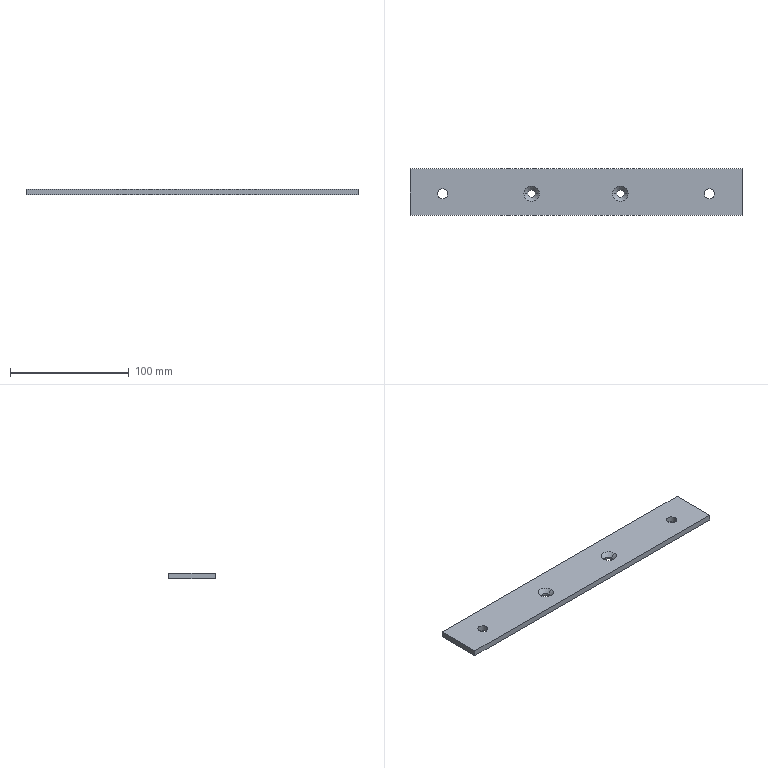Part | STEP file | 44-02-06 Ear Forming Push Plate A | 1 solid | 18 faces | box 280 x 39 x 5 mm | volume 53413 mm3 | cylinder 8 | plane 6 | cone 4 | commonest cylinder face diameters 6.5 x4 8.5 x4
STEP:
#1=CARTESIAN_POINT('',(0.,0.,0.));
#2=DIRECTION('',(0.,0.,1.));
#3=DIRECTION('',(1.,0.,0.));
#4=AXIS2_PLACEMENT_3D('',#1,#2,#3);
#5=CARTESIAN_POINT('',(-34.25,0.,-0.75));
#6=VERTEX_POINT('',#5);
#7=CARTESIAN_POINT('',(-31.,0.,2.5));
#8=VERTEX_POINT('',#7);
#9=CARTESIAN_POINT('',(-31.,0.,2.5));
#10=DIRECTION('',(0.7071,0.,0.7071));
#11=VECTOR('',#10,1.);
#12=LINE('',#9,#11);
#13=CARTESIAN_POINT('',(-37.5,0.,2.5));
#14=DIRECTION('',(0.,0.,1.));
#15=DIRECTION('',(1.,0.,0.));
#16=AXIS2_PLACEMENT_3D('',#13,#14,#15);
#17=CONICAL_SURFACE('',#16,6.5,0.7854);
#18=CARTESIAN_POINT('',(6.283,0.));
#19=DIRECTION('',(0.,1.));
#20=VECTOR('',#19,1.);
#21=LINE('',#18,#20);
#22=(GEOMETRIC_REPRESENTATION_CONTEXT(2)PARAMETRIC_REPRESENTATION_CONTEXT()REPRESENTATION_CONTEXT('',''));
#23=DEFINITIONAL_REPRESENTATION('',(#21),#22);
#24=PCURVE('',#17,#23);
#25=CARTESIAN_POINT('',(-37.5,0.,2.5));
#26=DIRECTION('',(0.,0.,1.));
#27=DIRECTION('',(1.,0.,0.));
#28=AXIS2_PLACEMENT_3D('',#25,#26,#27);
#29=CONICAL_SURFACE('',#28,6.5,0.7854);
#30=CARTESIAN_POINT('',(0.,0.));
#31=DIRECTION('',(0.,1.));
#32=VECTOR('',#31,1.);
#33=LINE('',#30,#32);
#34=(GEOMETRIC_REPRESENTATION_CONTEXT(2)PARAMETRIC_REPRESENTATION_CONTEXT()REPRESENTATION_CONTEXT('',''));
#35=DEFINITIONAL_REPRESENTATION('',(#33),#34);
#36=PCURVE('',#29,#35);
#37=SURFACE_CURVE('',#12,(#24,#36),.PCURVE_S1.);
#38=EDGE_CURVE('',#6,#8,#37,.T.);
#39=ORIENTED_EDGE('',*,*,#38,.T.);
#40=CARTESIAN_POINT('',(-44.,0.,2.5));
#41=VERTEX_POINT('',#40);
#42=CARTESIAN_POINT('',(-37.5,0.,2.5));
#43=DIRECTION('',(0.,0.,1.));
#44=DIRECTION('',(1.,0.,0.));
#45=AXIS2_PLACEMENT_3D('',#42,#43,#44);
#46=CIRCLE('',#45,6.5);
#47=CARTESIAN_POINT('',(0.,0.));
#48=DIRECTION('',(1.,0.));
#49=VECTOR('',#48,1.);
#50=LINE('',#47,#49);
#51=(GEOMETRIC_REPRESENTATION_CONTEXT(2)PARAMETRIC_REPRESENTATION_CONTEXT()REPRESENTATION_CONTEXT('',''));
#52=DEFINITIONAL_REPRESENTATION('',(#50),#51);
#53=PCURVE('',#17,#52);
#54=CARTESIAN_POINT('',(140.,-18.,2.5));
#55=DIRECTION('',(0.,0.,1.));
#56=DIRECTION('',(1.,0.,0.));
#57=AXIS2_PLACEMENT_3D('',#54,#55,#56);
#58=PLANE('',#57);
#59=CARTESIAN_POINT('',(-177.5,18.));
#60=DIRECTION('',(1.,0.));
#61=AXIS2_PLACEMENT_2D('',#59,#60);
#62=CIRCLE('',#61,6.5);
#63=(GEOMETRIC_REPRESENTATION_CONTEXT(2)PARAMETRIC_REPRESENTATION_CONTEXT()REPRESENTATION_CONTEXT('',''));
#64=DEFINITIONAL_REPRESENTATION('',(#62),#63);
#65=PCURVE('',#58,#64);
#66=SURFACE_CURVE('',#46,(#53,#65),.PCURVE_S1.);
#67=EDGE_CURVE('',#41,#8,#66,.T.);
#68=ORIENTED_EDGE('',*,*,#67,.F.);
#69=CARTESIAN_POINT('',(-40.75,0.,-0.75));
#70=VERTEX_POINT('',#69);
#71=CARTESIAN_POINT('',(-44.,0.,2.5));
#72=DIRECTION('',(-0.7071,0.,0.7071));
#73=VECTOR('',#72,1.);
#74=LINE('',#71,#73);
#75=CARTESIAN_POINT('',(3.142,0.));
#76=DIRECTION('',(0.,1.));
#77=VECTOR('',#76,1.);
#78=LINE('',#75,#77);
#79=(GEOMETRIC_REPRESENTATION_CONTEXT(2)PARAMETRIC_REPRESENTATION_CONTEXT()REPRESENTATION_CONTEXT('',''));
#80=DEFINITIONAL_REPRESENTATION('',(#78),#79);
#81=PCURVE('',#17,#80);
#82=CARTESIAN_POINT('',(3.142,0.));
#83=DIRECTION('',(0.,1.));
#84=VECTOR('',#83,1.);
#85=LINE('',#82,#84);
#86=(GEOMETRIC_REPRESENTATION_CONTEXT(2)PARAMETRIC_REPRESENTATION_CONTEXT()REPRESENTATION_CONTEXT('',''));
#87=DEFINITIONAL_REPRESENTATION('',(#85),#86);
#88=PCURVE('',#29,#87);
#89=SURFACE_CURVE('',#74,(#81,#88),.PCURVE_S1.);
#90=EDGE_CURVE('',#70,#41,#89,.T.);
#91=ORIENTED_EDGE('',*,*,#90,.F.);
#92=CARTESIAN_POINT('',(-37.5,0.,-0.75));
#93=DIRECTION('',(0.,0.,1.));
#94=DIRECTION('',(1.,0.,0.));
#95=AXIS2_PLACEMENT_3D('',#92,#93,#94);
#96=CIRCLE('',#95,3.25);
#97=CARTESIAN_POINT('',(0.,-3.25));
#98=DIRECTION('',(1.,0.));
#99=VECTOR('',#98,1.);
#100=LINE('',#97,#99);
#101=(GEOMETRIC_REPRESENTATION_CONTEXT(2)PARAMETRIC_REPRESENTATION_CONTEXT()REPRESENTATION_CONTEXT('',''));
#102=DEFINITIONAL_REPRESENTATION('',(#100),#101);
#103=PCURVE('',#17,#102);
#104=CARTESIAN_POINT('',(-37.5,0.,2.5));
#105=DIRECTION('',(0.,0.,1.));
#106=DIRECTION('',(1.,0.,0.));
#107=AXIS2_PLACEMENT_3D('',#104,#105,#106);
#108=CYLINDRICAL_SURFACE('',#107,3.25);
#109=CARTESIAN_POINT('',(0.,-3.25));
#110=DIRECTION('',(1.,0.));
#111=VECTOR('',#110,1.);
#112=LINE('',#109,#111);
#113=(GEOMETRIC_REPRESENTATION_CONTEXT(2)PARAMETRIC_REPRESENTATION_CONTEXT()REPRESENTATION_CONTEXT('',''));
#114=DEFINITIONAL_REPRESENTATION('',(#112),#113);
#115=PCURVE('',#108,#114);
#116=SURFACE_CURVE('',#96,(#103,#115),.PCURVE_S1.);
#117=EDGE_CURVE('',#70,#6,#116,.T.);
#118=ORIENTED_EDGE('',*,*,#117,.T.);
#119=EDGE_LOOP('',(#39,#68,#91,#118));
#120=FACE_BOUND('',#119,.F.);
#121=ADVANCED_FACE('',(#120),#17,.F.);
#122=CARTESIAN_POINT('',(-34.25,0.,-2.5));
#123=VERTEX_POINT('',#122);
#124=CARTESIAN_POINT('',(-34.25,0.,2.5));
#125=DIRECTION('',(0.,0.,1.));
#126=VECTOR('',#125,1.);
#127=LINE('',#124,#126);
#128=CARTESIAN_POINT('',(6.283,0.));
#129=DIRECTION('',(0.,1.));
#130=VECTOR('',#129,1.);
#131=LINE('',#128,#130);
#132=(GEOMETRIC_REPRESENTATION_CONTEXT(2)PARAMETRIC_REPRESENTATION_CONTEXT()REPRESENTATION_CONTEXT('',''));
#133=DEFINITIONAL_REPRESENTATION('',(#131),#132);
#134=PCURVE('',#108,#133);
#135=CARTESIAN_POINT('',(-37.5,0.,2.5));
#136=DIRECTION('',(0.,0.,1.));
#137=DIRECTION('',(1.,0.,0.));
#138=AXIS2_PLACEMENT_3D('',#135,#136,#137);
#139=CYLINDRICAL_SURFACE('',#138,3.25);
#140=CARTESIAN_POINT('',(0.,0.));
#141=DIRECTION('',(0.,1.));
#142=VECTOR('',#141,1.);
#143=LINE('',#140,#142);
#144=(GEOMETRIC_REPRESENTATION_CONTEXT(2)PARAMETRIC_REPRESENTATION_CONTEXT()REPRESENTATION_CONTEXT('',''));
#145=DEFINITIONAL_REPRESENTATION('',(#143),#144);
#146=PCURVE('',#139,#145);
#147=SURFACE_CURVE('',#127,(#134,#146),.PCURVE_S1.);
#148=EDGE_CURVE('',#123,#6,#147,.T.);
#149=ORIENTED_EDGE('',*,*,#148,.T.);
#150=ORIENTED_EDGE('',*,*,#117,.F.);
#151=CARTESIAN_POINT('',(-40.75,0.,-2.5));
#152=VERTEX_POINT('',#151);
#153=CARTESIAN_POINT('',(-40.75,0.,2.5));
#154=DIRECTION('',(0.,0.,1.));
#155=VECTOR('',#154,1.);
#156=LINE('',#153,#155);
#157=CARTESIAN_POINT('',(3.142,0.));
#158=DIRECTION('',(0.,1.));
#159=VECTOR('',#158,1.);
#160=LINE('',#157,#159);
#161=(GEOMETRIC_REPRESENTATION_CONTEXT(2)PARAMETRIC_REPRESENTATION_CONTEXT()REPRESENTATION_CONTEXT('',''));
#162=DEFINITIONAL_REPRESENTATION('',(#160),#161);
#163=PCURVE('',#108,#162);
#164=CARTESIAN_POINT('',(3.142,0.));
#165=DIRECTION('',(0.,1.));
#166=VECTOR('',#165,1.);
#167=LINE('',#164,#166);
#168=(GEOMETRIC_REPRESENTATION_CONTEXT(2)PARAMETRIC_REPRESENTATION_CONTEXT()REPRESENTATION_CONTEXT('',''));
#169=DEFINITIONAL_REPRESENTATION('',(#167),#168);
#170=PCURVE('',#139,#169);
#171=SURFACE_CURVE('',#156,(#163,#170),.PCURVE_S1.);
#172=EDGE_CURVE('',#152,#70,#171,.T.);
#173=ORIENTED_EDGE('',*,*,#172,.F.);
#174=CARTESIAN_POINT('',(-37.5,0.,-2.5));
#175=DIRECTION('',(0.,0.,1.));
#176=DIRECTION('',(1.,0.,0.));
#177=AXIS2_PLACEMENT_3D('',#174,#175,#176);
#178=CIRCLE('',#177,3.25);
#179=CARTESIAN_POINT('',(0.,-5.));
#180=DIRECTION('',(1.,0.));
#181=VECTOR('',#180,1.);
#182=LINE('',#179,#181);
#183=(GEOMETRIC_REPRESENTATION_CONTEXT(2)PARAMETRIC_REPRESENTATION_CONTEXT()REPRESENTATION_CONTEXT('',''));
#184=DEFINITIONAL_REPRESENTATION('',(#182),#183);
#185=PCURVE('',#108,#184);
#186=CARTESIAN_POINT('',(140.,-18.,-2.5));
#187=DIRECTION('',(0.,0.,1.));
#188=DIRECTION('',(1.,0.,0.));
#189=AXIS2_PLACEMENT_3D('',#186,#187,#188);
#190=PLANE('',#189);
#191=CARTESIAN_POINT('',(-177.5,18.));
#192=DIRECTION('',(1.,0.));
#193=AXIS2_PLACEMENT_2D('',#191,#192);
#194=CIRCLE('',#193,3.25);
#195=(GEOMETRIC_REPRESENTATION_CONTEXT(2)PARAMETRIC_REPRESENTATION_CONTEXT()REPRESENTATION_CONTEXT('',''));
#196=DEFINITIONAL_REPRESENTATION('',(#194),#195);
#197=PCURVE('',#190,#196);
#198=SURFACE_CURVE('',#178,(#185,#197),.PCURVE_S1.);
#199=EDGE_CURVE('',#152,#123,#198,.T.);
#200=ORIENTED_EDGE('',*,*,#199,.T.);
#201=EDGE_LOOP('',(#149,#150,#173,#200));
#202=FACE_BOUND('',#201,.F.);
#203=ADVANCED_FACE('',(#202),#108,.F.);
#204=CARTESIAN_POINT('',(40.75,0.,-0.75));
#205=VERTEX_POINT('',#204);
#206=CARTESIAN_POINT('',(44.,0.,2.5));
#207=VERTEX_POINT('',#206);
#208=CARTESIAN_POINT('',(44.,0.,2.5));
#209=DIRECTION('',(0.7071,0.,0.7071));
#210=VECTOR('',#209,1.);
#211=LINE('',#208,#210);
#212=CARTESIAN_POINT('',(37.5,0.,2.5));
#213=DIRECTION('',(0.,0.,1.));
#214=DIRECTION('',(1.,0.,0.));
#215=AXIS2_PLACEMENT_3D('',#212,#213,#214);
#216=CONICAL_SURFACE('',#215,6.5,0.7854);
#217=CARTESIAN_POINT('',(6.283,0.));
#218=DIRECTION('',(0.,1.));
#219=VECTOR('',#218,1.);
#220=LINE('',#217,#219);
#221=(GEOMETRIC_REPRESENTATION_CONTEXT(2)PARAMETRIC_REPRESENTATION_CONTEXT()REPRESENTATION_CONTEXT('',''));
#222=DEFINITIONAL_REPRESENTATION('',(#220),#221);
#223=PCURVE('',#216,#222);
#224=CARTESIAN_POINT('',(37.5,0.,2.5));
#225=DIRECTION('',(0.,0.,1.));
#226=DIRECTION('',(1.,0.,0.));
#227=AXIS2_PLACEMENT_3D('',#224,#225,#226);
#228=CONICAL_SURFACE('',#227,6.5,0.7854);
#229=CARTESIAN_POINT('',(0.,0.));
#230=DIRECTION('',(0.,1.));
#231=VECTOR('',#230,1.);
#232=LINE('',#229,#231);
#233=(GEOMETRIC_REPRESENTATION_CONTEXT(2)PARAMETRIC_REPRESENTATION_CONTEXT()REPRESENTATION_CONTEXT('',''));
#234=DEFINITIONAL_REPRESENTATION('',(#232),#233);
#235=PCURVE('',#228,#234);
#236=SURFACE_CURVE('',#211,(#223,#235),.PCURVE_S1.);
#237=EDGE_CURVE('',#205,#207,#236,.T.);
#238=ORIENTED_EDGE('',*,*,#237,.T.);
#239=CARTESIAN_POINT('',(31.,0.,2.5));
#240=VERTEX_POINT('',#239);
#241=CARTESIAN_POINT('',(37.5,0.,2.5));
#242=DIRECTION('',(0.,0.,1.));
#243=DIRECTION('',(1.,0.,0.));
#244=AXIS2_PLACEMENT_3D('',#241,#242,#243);
#245=CIRCLE('',#244,6.5);
#246=CARTESIAN_POINT('',(0.,0.));
#247=DIRECTION('',(1.,0.));
#248=VECTOR('',#247,1.);
#249=LINE('',#246,#248);
#250=(GEOMETRIC_REPRESENTATION_CONTEXT(2)PARAMETRIC_REPRESENTATION_CONTEXT()REPRESENTATION_CONTEXT('',''));
#251=DEFINITIONAL_REPRESENTATION('',(#249),#250);
#252=PCURVE('',#216,#251);
#253=CARTESIAN_POINT('',(-102.5,18.));
#254=DIRECTION('',(1.,0.));
#255=AXIS2_PLACEMENT_2D('',#253,#254);
#256=CIRCLE('',#255,6.5);
#257=(GEOMETRIC_REPRESENTATION_CONTEXT(2)PARAMETRIC_REPRESENTATION_CONTEXT()REPRESENTATION_CONTEXT('',''));
#258=DEFINITIONAL_REPRESENTATION('',(#256),#257);
#259=PCURVE('',#58,#258);
#260=SURFACE_CURVE('',#245,(#252,#259),.PCURVE_S1.);
#261=EDGE_CURVE('',#240,#207,#260,.T.);
#262=ORIENTED_EDGE('',*,*,#261,.F.);
#263=CARTESIAN_POINT('',(34.25,0.,-0.75));
#264=VERTEX_POINT('',#263);
#265=CARTESIAN_POINT('',(31.,0.,2.5));
#266=DIRECTION('',(-0.7071,0.,0.7071));
#267=VECTOR('',#266,1.);
#268=LINE('',#265,#267);
#269=CARTESIAN_POINT('',(3.142,0.));
#270=DIRECTION('',(0.,1.));
#271=VECTOR('',#270,1.);
#272=LINE('',#269,#271);
#273=(GEOMETRIC_REPRESENTATION_CONTEXT(2)PARAMETRIC_REPRESENTATION_CONTEXT()REPRESENTATION_CONTEXT('',''));
#274=DEFINITIONAL_REPRESENTATION('',(#272),#273);
#275=PCURVE('',#216,#274);
#276=CARTESIAN_POINT('',(3.142,0.));
#277=DIRECTION('',(0.,1.));
#278=VECTOR('',#277,1.);
#279=LINE('',#276,#278);
#280=(GEOMETRIC_REPRESENTATION_CONTEXT(2)PARAMETRIC_REPRESENTATION_CONTEXT()REPRESENTATION_CONTEXT('',''));
#281=DEFINITIONAL_REPRESENTATION('',(#279),#280);
#282=PCURVE('',#228,#281);
#283=SURFACE_CURVE('',#268,(#275,#282),.PCURVE_S1.);
#284=EDGE_CURVE('',#264,#240,#283,.T.);
#285=ORIENTED_EDGE('',*,*,#284,.F.);
#286=CARTESIAN_POINT('',(37.5,0.,-0.75));
#287=DIRECTION('',(0.,0.,1.));
#288=DIRECTION('',(1.,0.,0.));
#289=AXIS2_PLACEMENT_3D('',#286,#287,#288);
#290=CIRCLE('',#289,3.25);
#291=CARTESIAN_POINT('',(0.,-3.25));
#292=DIRECTION('',(1.,0.));
#293=VECTOR('',#292,1.);
#294=LINE('',#291,#293);
#295=(GEOMETRIC_REPRESENTATION_CONTEXT(2)PARAMETRIC_REPRESENTATION_CONTEXT()REPRESENTATION_CONTEXT('',''));
#296=DEFINITIONAL_REPRESENTATION('',(#294),#295);
#297=PCURVE('',#216,#296);
#298=CARTESIAN_POINT('',(37.5,0.,2.5));
#299=DIRECTION('',(0.,0.,1.));
#300=DIRECTION('',(1.,0.,0.));
#301=AXIS2_PLACEMENT_3D('',#298,#299,#300);
#302=CYLINDRICAL_SURFACE('',#301,3.25);
#303=CARTESIAN_POINT('',(0.,-3.25));
#304=DIRECTION('',(1.,0.));
#305=VECTOR('',#304,1.);
#306=LINE('',#303,#305);
#307=(GEOMETRIC_REPRESENTATION_CONTEXT(2)PARAMETRIC_REPRESENTATION_CONTEXT()REPRESENTATION_CONTEXT('',''));
#308=DEFINITIONAL_REPRESENTATION('',(#306),#307);
#309=PCURVE('',#302,#308);
#310=SURFACE_CURVE('',#290,(#297,#309),.PCURVE_S1.);
#311=EDGE_CURVE('',#264,#205,#310,.T.);
#312=ORIENTED_EDGE('',*,*,#311,.T.);
#313=EDGE_LOOP('',(#238,#262,#285,#312));
#314=FACE_BOUND('',#313,.F.);
#315=ADVANCED_FACE('',(#314),#216,.F.);
#316=CARTESIAN_POINT('',(40.75,0.,-2.5));
#317=VERTEX_POINT('',#316);
#318=CARTESIAN_POINT('',(40.75,0.,2.5));
#319=DIRECTION('',(0.,0.,1.));
#320=VECTOR('',#319,1.);
#321=LINE('',#318,#320);
#322=CARTESIAN_POINT('',(6.283,0.));
#323=DIRECTION('',(0.,1.));
#324=VECTOR('',#323,1.);
#325=LINE('',#322,#324);
#326=(GEOMETRIC_REPRESENTATION_CONTEXT(2)PARAMETRIC_REPRESENTATION_CONTEXT()REPRESENTATION_CONTEXT('',''));
#327=DEFINITIONAL_REPRESENTATION('',(#325),#326);
#328=PCURVE('',#302,#327);
#329=CARTESIAN_POINT('',(37.5,0.,2.5));
#330=DIRECTION('',(0.,0.,1.));
#331=DIRECTION('',(1.,0.,0.));
#332=AXIS2_PLACEMENT_3D('',#329,#330,#331);
#333=CYLINDRICAL_SURFACE('',#332,3.25);
#334=CARTESIAN_POINT('',(0.,0.));
#335=DIRECTION('',(0.,1.));
#336=VECTOR('',#335,1.);
#337=LINE('',#334,#336);
#338=(GEOMETRIC_REPRESENTATION_CONTEXT(2)PARAMETRIC_REPRESENTATION_CONTEXT()REPRESENTATION_CONTEXT('',''));
#339=DEFINITIONAL_REPRESENTATION('',(#337),#338);
#340=PCURVE('',#333,#339);
#341=SURFACE_CURVE('',#321,(#328,#340),.PCURVE_S1.);
#342=EDGE_CURVE('',#317,#205,#341,.T.);
#343=ORIENTED_EDGE('',*,*,#342,.T.);
#344=ORIENTED_EDGE('',*,*,#311,.F.);
#345=CARTESIAN_POINT('',(34.25,0.,-2.5));
#346=VERTEX_POINT('',#345);
#347=CARTESIAN_POINT('',(34.25,0.,2.5));
#348=DIRECTION('',(0.,0.,1.));
#349=VECTOR('',#348,1.);
#350=LINE('',#347,#349);
#351=CARTESIAN_POINT('',(3.142,0.));
#352=DIRECTION('',(0.,1.));
#353=VECTOR('',#352,1.);
#354=LINE('',#351,#353);
#355=(GEOMETRIC_REPRESENTATION_CONTEXT(2)PARAMETRIC_REPRESENTATION_CONTEXT()REPRESENTATION_CONTEXT('',''));
#356=DEFINITIONAL_REPRESENTATION('',(#354),#355);
#357=PCURVE('',#302,#356);
#358=CARTESIAN_POINT('',(3.142,0.));
#359=DIRECTION('',(0.,1.));
#360=VECTOR('',#359,1.);
#361=LINE('',#358,#360);
#362=(GEOMETRIC_REPRESENTATION_CONTEXT(2)PARAMETRIC_REPRESENTATION_CONTEXT()REPRESENTATION_CONTEXT('',''));
#363=DEFINITIONAL_REPRESENTATION('',(#361),#362);
#364=PCURVE('',#333,#363);
#365=SURFACE_CURVE('',#350,(#357,#364),.PCURVE_S1.);
#366=EDGE_CURVE('',#346,#264,#365,.T.);
#367=ORIENTED_EDGE('',*,*,#366,.F.);
#368=CARTESIAN_POINT('',(37.5,0.,-2.5));
#369=DIRECTION('',(0.,0.,1.));
#370=DIRECTION('',(1.,0.,0.));
#371=AXIS2_PLACEMENT_3D('',#368,#369,#370);
#372=CIRCLE('',#371,3.25);
#373=CARTESIAN_POINT('',(0.,-5.));
#374=DIRECTION('',(1.,0.));
#375=VECTOR('',#374,1.);
#376=LINE('',#373,#375);
#377=(GEOMETRIC_REPRESENTATION_CONTEXT(2)PARAMETRIC_REPRESENTATION_CONTEXT()REPRESENTATION_CONTEXT('',''));
#378=DEFINITIONAL_REPRESENTATION('',(#376),#377);
#379=PCURVE('',#302,#378);
#380=CARTESIAN_POINT('',(-102.5,18.));
#381=DIRECTION('',(1.,0.));
#382=AXIS2_PLACEMENT_2D('',#380,#381);
#383=CIRCLE('',#382,3.25);
#384=(GEOMETRIC_REPRESENTATION_CONTEXT(2)PARAMETRIC_REPRESENTATION_CONTEXT()REPRESENTATION_CONTEXT('',''));
#385=DEFINITIONAL_REPRESENTATION('',(#383),#384);
#386=PCURVE('',#190,#385);
#387=SURFACE_CURVE('',#372,(#379,#386),.PCURVE_S1.);
#388=EDGE_CURVE('',#346,#317,#387,.T.);
#389=ORIENTED_EDGE('',*,*,#388,.T.);
#390=EDGE_LOOP('',(#343,#344,#367,#389));
#391=FACE_BOUND('',#390,.F.);
#392=ADVANCED_FACE('',(#391),#302,.F.);
#393=CARTESIAN_POINT('',(108.25,0.,2.5));
#394=VERTEX_POINT('',#393);
#395=CARTESIAN_POINT('',(108.25,0.,-2.5));
#396=VERTEX_POINT('',#395);
#397=CARTESIAN_POINT('',(108.25,0.,-2.5));
#398=DIRECTION('',(0.,0.,-1.));
#399=VECTOR('',#398,1.);
#400=LINE('',#397,#399);
#401=CARTESIAN_POINT('',(112.5,0.,-2.5));
#402=DIRECTION('',(0.,0.,-1.));
#403=DIRECTION('',(-1.,0.,0.));
#404=AXIS2_PLACEMENT_3D('',#401,#402,#403);
#405=CYLINDRICAL_SURFACE('',#404,4.25);
#406=CARTESIAN_POINT('',(6.283,0.));
#407=DIRECTION('',(0.,1.));
#408=VECTOR('',#407,1.);
#409=LINE('',#406,#408);
#410=(GEOMETRIC_REPRESENTATION_CONTEXT(2)PARAMETRIC_REPRESENTATION_CONTEXT()REPRESENTATION_CONTEXT('',''));
#411=DEFINITIONAL_REPRESENTATION('',(#409),#410);
#412=PCURVE('',#405,#411);
#413=CARTESIAN_POINT('',(112.5,0.,-2.5));
#414=DIRECTION('',(0.,0.,-1.));
#415=DIRECTION('',(-1.,0.,0.));
#416=AXIS2_PLACEMENT_3D('',#413,#414,#415);
#417=CYLINDRICAL_SURFACE('',#416,4.25);
#418=CARTESIAN_POINT('',(0.,0.));
#419=DIRECTION('',(0.,1.));
#420=VECTOR('',#419,1.);
#421=LINE('',#418,#420);
#422=(GEOMETRIC_REPRESENTATION_CONTEXT(2)PARAMETRIC_REPRESENTATION_CONTEXT()REPRESENTATION_CONTEXT('',''));
#423=DEFINITIONAL_REPRESENTATION('',(#421),#422);
#424=PCURVE('',#417,#423);
#425=SURFACE_CURVE('',#400,(#412,#424),.PCURVE_S1.);
#426=EDGE_CURVE('',#394,#396,#425,.T.);
#427=ORIENTED_EDGE('',*,*,#426,.T.);
#428=CARTESIAN_POINT('',(116.75,0.,-2.5));
#429=VERTEX_POINT('',#428);
#430=CARTESIAN_POINT('',(112.5,0.,-2.5));
#431=DIRECTION('',(0.,0.,-1.));
#432=DIRECTION('',(-1.,0.,0.));
#433=AXIS2_PLACEMENT_3D('',#430,#431,#432);
#434=CIRCLE('',#433,4.25);
#435=CARTESIAN_POINT('',(0.,0.));
#436=DIRECTION('',(1.,0.));
#437=VECTOR('',#436,1.);
#438=LINE('',#435,#437);
#439=(GEOMETRIC_REPRESENTATION_CONTEXT(2)PARAMETRIC_REPRESENTATION_CONTEXT()REPRESENTATION_CONTEXT('',''));
#440=DEFINITIONAL_REPRESENTATION('',(#438),#439);
#441=PCURVE('',#405,#440);
#442=CARTESIAN_POINT('',(-31.75,18.));
#443=CARTESIAN_POINT('',(-31.75,25.361));
#444=CARTESIAN_POINT('',(-25.375,21.681));
#445=CARTESIAN_POINT('',(-19.,18.));
#446=CARTESIAN_POINT('',(-25.375,14.319));
#447=CARTESIAN_POINT('',(-31.75,10.639));
#448=CARTESIAN_POINT('',(-31.75,18.));
#449=(BOUNDED_CURVE()B_SPLINE_CURVE(2,(#442,#443,#444,#445,#446,#447,#448),.UNSPECIFIED.,.T.,.F.)B_SPLINE_CURVE_WITH_KNOTS((1,2,2,2,2,1),(-2.094,0.,2.094,4.189,6.283,8.378),.UNSPECIFIED.)CURVE()GEOMETRIC_REPRESENTATION_ITEM()RATIONAL_B_SPLINE_CURVE((1.,0.5,1.,0.5,1.,0.5,1.))REPRESENTATION_ITEM(''));
#450=(GEOMETRIC_REPRESENTATION_CONTEXT(2)PARAMETRIC_REPRESENTATION_CONTEXT()REPRESENTATION_CONTEXT('',''));
#451=DEFINITIONAL_REPRESENTATION('',(#449),#450);
#452=PCURVE('',#190,#451);
#453=SURFACE_CURVE('',#434,(#441,#452),.PCURVE_S1.);
#454=EDGE_CURVE('',#429,#396,#453,.T.);
#455=ORIENTED_EDGE('',*,*,#454,.F.);
#456=CARTESIAN_POINT('',(116.75,0.,2.5));
#457=VERTEX_POINT('',#456);
#458=CARTESIAN_POINT('',(116.75,0.,-2.5));
#459=DIRECTION('',(0.,0.,-1.));
#460=VECTOR('',#459,1.);
#461=LINE('',#458,#460);
#462=CARTESIAN_POINT('',(3.142,0.));
#463=DIRECTION('',(0.,1.));
#464=VECTOR('',#463,1.);
#465=LINE('',#462,#464);
#466=(GEOMETRIC_REPRESENTATION_CONTEXT(2)PARAMETRIC_REPRESENTATION_CONTEXT()REPRESENTATION_CONTEXT('',''));
#467=DEFINITIONAL_REPRESENTATION('',(#465),#466);
#468=PCURVE('',#405,#467);
#469=CARTESIAN_POINT('',(3.142,0.));
#470=DIRECTION('',(0.,1.));
#471=VECTOR('',#470,1.);
#472=LINE('',#469,#471);
#473=(GEOMETRIC_REPRESENTATION_CONTEXT(2)PARAMETRIC_REPRESENTATION_CONTEXT()REPRESENTATION_CONTEXT('',''));
#474=DEFINITIONAL_REPRESENTATION('',(#472),#473);
#475=PCURVE('',#417,#474);
#476=SURFACE_CURVE('',#461,(#468,#475),.PCURVE_S1.);
#477=EDGE_CURVE('',#457,#429,#476,.T.);
#478=ORIENTED_EDGE('',*,*,#477,.F.);
#479=CARTESIAN_POINT('',(112.5,0.,2.5));
#480=DIRECTION('',(0.,0.,1.));
#481=DIRECTION('',(1.,0.,0.));
#482=AXIS2_PLACEMENT_3D('',#479,#480,#481);
#483=CIRCLE('',#482,4.25);
#484=CARTESIAN_POINT('',(9.425,-5.));
#485=DIRECTION('',(-1.,0.));
#486=VECTOR('',#485,1.);
#487=LINE('',#484,#486);
#488=(GEOMETRIC_REPRESENTATION_CONTEXT(2)PARAMETRIC_REPRESENTATION_CONTEXT()REPRESENTATION_CONTEXT('',''));
#489=DEFINITIONAL_REPRESENTATION('',(#487),#488);
#490=PCURVE('',#405,#489);
#491=CARTESIAN_POINT('',(-27.5,18.));
#492=DIRECTION('',(1.,0.));
#493=AXIS2_PLACEMENT_2D('',#491,#492);
#494=CIRCLE('',#493,4.25);
#495=(GEOMETRIC_REPRESENTATION_CONTEXT(2)PARAMETRIC_REPRESENTATION_CONTEXT()REPRESENTATION_CONTEXT('',''));
#496=DEFINITIONAL_REPRESENTATION('',(#494),#495);
#497=PCURVE('',#58,#496);
#498=SURFACE_CURVE('',#483,(#490,#497),.PCURVE_S1.);
#499=EDGE_CURVE('',#394,#457,#498,.T.);
#500=ORIENTED_EDGE('',*,*,#499,.F.);
#501=EDGE_LOOP('',(#427,#455,#478,#500));
#502=FACE_BOUND('',#501,.F.);
#503=ADVANCED_FACE('',(#502),#405,.F.);
#504=CARTESIAN_POINT('',(-116.75,0.,2.5));
#505=VERTEX_POINT('',#504);
#506=CARTESIAN_POINT('',(-116.75,0.,-2.5));
#507=VERTEX_POINT('',#506);
#508=CARTESIAN_POINT('',(-116.75,0.,-2.5));
#509=DIRECTION('',(0.,0.,-1.));
#510=VECTOR('',#509,1.);
#511=LINE('',#508,#510);
#512=CARTESIAN_POINT('',(-112.5,0.,-2.5));
#513=DIRECTION('',(0.,0.,-1.));
#514=DIRECTION('',(-1.,0.,0.));
#515=AXIS2_PLACEMENT_3D('',#512,#513,#514);
#516=CYLINDRICAL_SURFACE('',#515,4.25);
#517=CARTESIAN_POINT('',(6.283,0.));
#518=DIRECTION('',(0.,1.));
#519=VECTOR('',#518,1.);
#520=LINE('',#517,#519);
#521=(GEOMETRIC_REPRESENTATION_CONTEXT(2)PARAMETRIC_REPRESENTATION_CONTEXT()REPRESENTATION_CONTEXT('',''));
#522=DEFINITIONAL_REPRESENTATION('',(#520),#521);
#523=PCURVE('',#516,#522);
#524=CARTESIAN_POINT('',(-112.5,0.,-2.5));
#525=DIRECTION('',(0.,0.,-1.));
#526=DIRECTION('',(-1.,0.,0.));
#527=AXIS2_PLACEMENT_3D('',#524,#525,#526);
#528=CYLINDRICAL_SURFACE('',#527,4.25);
#529=CARTESIAN_POINT('',(0.,0.));
#530=DIRECTION('',(0.,1.));
#531=VECTOR('',#530,1.);
#532=LINE('',#529,#531);
#533=(GEOMETRIC_REPRESENTATION_CONTEXT(2)PARAMETRIC_REPRESENTATION_CONTEXT()REPRESENTATION_CONTEXT('',''));
#534=DEFINITIONAL_REPRESENTATION('',(#532),#533);
#535=PCURVE('',#528,#534);
#536=SURFACE_CURVE('',#511,(#523,#535),.PCURVE_S1.);
#537=EDGE_CURVE('',#505,#507,#536,.T.);
#538=ORIENTED_EDGE('',*,*,#537,.T.);
#539=CARTESIAN_POINT('',(-108.25,0.,-2.5));
#540=VERTEX_POINT('',#539);
#541=CARTESIAN_POINT('',(-112.5,0.,-2.5));
#542=DIRECTION('',(0.,0.,-1.));
#543=DIRECTION('',(-1.,0.,0.));
#544=AXIS2_PLACEMENT_3D('',#541,#542,#543);
#545=CIRCLE('',#544,4.25);
#546=CARTESIAN_POINT('',(0.,0.));
#547=DIRECTION('',(1.,0.));
#548=VECTOR('',#547,1.);
#549=LINE('',#546,#548);
#550=(GEOMETRIC_REPRESENTATION_CONTEXT(2)PARAMETRIC_REPRESENTATION_CONTEXT()REPRESENTATION_CONTEXT('',''));
#551=DEFINITIONAL_REPRESENTATION('',(#549),#550);
#552=PCURVE('',#516,#551);
#553=CARTESIAN_POINT('',(-256.75,18.));
#554=CARTESIAN_POINT('',(-256.75,25.361));
#555=CARTESIAN_POINT('',(-250.375,21.681));
#556=CARTESIAN_POINT('',(-244.,18.));
#557=CARTESIAN_POINT('',(-250.375,14.319));
#558=CARTESIAN_POINT('',(-256.75,10.639));
#559=CARTESIAN_POINT('',(-256.75,18.));
#560=(BOUNDED_CURVE()B_SPLINE_CURVE(2,(#553,#554,#555,#556,#557,#558,#559),.UNSPECIFIED.,.T.,.F.)B_SPLINE_CURVE_WITH_KNOTS((1,2,2,2,2,1),(-2.094,0.,2.094,4.189,6.283,8.378),.UNSPECIFIED.)CURVE()GEOMETRIC_REPRESENTATION_ITEM()RATIONAL_B_SPLINE_CURVE((1.,0.5,1.,0.5,1.,0.5,1.))REPRESENTATION_ITEM(''));
#561=(GEOMETRIC_REPRESENTATION_CONTEXT(2)PARAMETRIC_REPRESENTATION_CONTEXT()REPRESENTATION_CONTEXT('',''));
#562=DEFINITIONAL_REPRESENTATION('',(#560),#561);
#563=PCURVE('',#190,#562);
#564=SURFACE_CURVE('',#545,(#552,#563),.PCURVE_S1.);
#565=EDGE_CURVE('',#540,#507,#564,.T.);
#566=ORIENTED_EDGE('',*,*,#565,.F.);
#567=CARTESIAN_POINT('',(-108.25,0.,2.5));
#568=VERTEX_POINT('',#567);
#569=CARTESIAN_POINT('',(-108.25,0.,-2.5));
#570=DIRECTION('',(0.,0.,-1.));
#571=VECTOR('',#570,1.);
#572=LINE('',#569,#571);
#573=CARTESIAN_POINT('',(3.142,0.));
#574=DIRECTION('',(0.,1.));
#575=VECTOR('',#574,1.);
#576=LINE('',#573,#575);
#577=(GEOMETRIC_REPRESENTATION_CONTEXT(2)PARAMETRIC_REPRESENTATION_CONTEXT()REPRESENTATION_CONTEXT('',''));
#578=DEFINITIONAL_REPRESENTATION('',(#576),#577);
#579=PCURVE('',#516,#578);
#580=CARTESIAN_POINT('',(3.142,0.));
#581=DIRECTION('',(0.,1.));
#582=VECTOR('',#581,1.);
#583=LINE('',#580,#582);
#584=(GEOMETRIC_REPRESENTATION_CONTEXT(2)PARAMETRIC_REPRESENTATION_CONTEXT()REPRESENTATION_CONTEXT('',''));
#585=DEFINITIONAL_REPRESENTATION('',(#583),#584);
#586=PCURVE('',#528,#585);
#587=SURFACE_CURVE('',#572,(#579,#586),.PCURVE_S1.);
#588=EDGE_CURVE('',#568,#540,#587,.T.);
#589=ORIENTED_EDGE('',*,*,#588,.F.);
#590=CARTESIAN_POINT('',(-112.5,0.,2.5));
#591=DIRECTION('',(0.,0.,1.));
#592=DIRECTION('',(1.,0.,0.));
#593=AXIS2_PLACEMENT_3D('',#590,#591,#592);
#594=CIRCLE('',#593,4.25);
#595=CARTESIAN_POINT('',(9.425,-5.));
#596=DIRECTION('',(-1.,0.));
#597=VECTOR('',#596,1.);
#598=LINE('',#595,#597);
#599=(GEOMETRIC_REPRESENTATION_CONTEXT(2)PARAMETRIC_REPRESENTATION_CONTEXT()REPRESENTATION_CONTEXT('',''));
#600=DEFINITIONAL_REPRESENTATION('',(#598),#599);
#601=PCURVE('',#516,#600);
#602=CARTESIAN_POINT('',(-252.5,18.));
#603=DIRECTION('',(1.,0.));
#604=AXIS2_PLACEMENT_2D('',#602,#603);
#605=CIRCLE('',#604,4.25);
#606=(GEOMETRIC_REPRESENTATION_CONTEXT(2)PARAMETRIC_REPRESENTATION_CONTEXT()REPRESENTATION_CONTEXT('',''));
#607=DEFINITIONAL_REPRESENTATION('',(#605),#606);
#608=PCURVE('',#58,#607);
#609=SURFACE_CURVE('',#594,(#601,#608),.PCURVE_S1.);
#610=EDGE_CURVE('',#505,#568,#609,.T.);
#611=ORIENTED_EDGE('',*,*,#610,.F.);
#612=EDGE_LOOP('',(#538,#566,#589,#611));
#613=FACE_BOUND('',#612,.F.);
#614=ADVANCED_FACE('',(#613),#516,.F.);
#615=CARTESIAN_POINT('',(140.,-18.,-2.5));
#616=VERTEX_POINT('',#615);
#617=CARTESIAN_POINT('',(140.,21.,-2.5));
#618=VERTEX_POINT('',#617);
#619=CARTESIAN_POINT('',(140.,18.,-2.5));
#620=DIRECTION('',(0.,1.,0.));
#621=VECTOR('',#620,1.);
#622=LINE('',#619,#621);
#623=CARTESIAN_POINT('',(140.,18.,2.5));
#624=DIRECTION('',(-1.,0.,0.));
#625=DIRECTION('',(0.,0.,1.));
#626=AXIS2_PLACEMENT_3D('',#623,#624,#625);
#627=PLANE('',#626);
#628=CARTESIAN_POINT('',(-5.,0.));
#629=DIRECTION('',(0.,1.));
#630=VECTOR('',#629,1.);
#631=LINE('',#628,#630);
#632=(GEOMETRIC_REPRESENTATION_CONTEXT(2)PARAMETRIC_REPRESENTATION_CONTEXT()REPRESENTATION_CONTEXT('',''));
#633=DEFINITIONAL_REPRESENTATION('',(#631),#632);
#634=PCURVE('',#627,#633);
#635=CARTESIAN_POINT('',(0.,36.));
#636=DIRECTION('',(0.,1.));
#637=VECTOR('',#636,1.);
#638=LINE('',#635,#637);
#639=(GEOMETRIC_REPRESENTATION_CONTEXT(2)PARAMETRIC_REPRESENTATION_CONTEXT()REPRESENTATION_CONTEXT('',''));
#640=DEFINITIONAL_REPRESENTATION('',(#638),#639);
#641=PCURVE('',#190,#640);
#642=SURFACE_CURVE('',#622,(#634,#641),.PCURVE_S1.);
#643=EDGE_CURVE('',#616,#618,#642,.T.);
#644=ORIENTED_EDGE('',*,*,#643,.T.);
#645=CARTESIAN_POINT('',(140.,21.,2.5));
#646=VERTEX_POINT('',#645);
#647=CARTESIAN_POINT('',(140.,21.,2.5));
#648=DIRECTION('',(0.,0.,1.));
#649=VECTOR('',#648,1.);
#650=LINE('',#647,#649);
#651=CARTESIAN_POINT('',(0.,3.));
#652=DIRECTION('',(1.,0.));
#653=VECTOR('',#652,1.);
#654=LINE('',#651,#653);
#655=(GEOMETRIC_REPRESENTATION_CONTEXT(2)PARAMETRIC_REPRESENTATION_CONTEXT()REPRESENTATION_CONTEXT('',''));
#656=DEFINITIONAL_REPRESENTATION('',(#654),#655);
#657=PCURVE('',#627,#656);
#658=CARTESIAN_POINT('',(-140.,21.,-2.5));
#659=DIRECTION('',(0.,-1.,0.));
#660=DIRECTION('',(0.,0.,-1.));
#661=AXIS2_PLACEMENT_3D('',#658,#659,#660);
#662=PLANE('',#661);
#663=CARTESIAN_POINT('',(-5.,280.));
#664=DIRECTION('',(-1.,0.));
#665=VECTOR('',#664,1.);
#666=LINE('',#663,#665);
#667=(GEOMETRIC_REPRESENTATION_CONTEXT(2)PARAMETRIC_REPRESENTATION_CONTEXT()REPRESENTATION_CONTEXT('',''));
#668=DEFINITIONAL_REPRESENTATION('',(#666),#667);
#669=PCURVE('',#662,#668);
#670=SURFACE_CURVE('',#650,(#657,#669),.PCURVE_S1.);
#671=EDGE_CURVE('',#618,#646,#670,.T.);
#672=ORIENTED_EDGE('',*,*,#671,.T.);
#673=CARTESIAN_POINT('',(140.,-18.,2.5));
#674=VERTEX_POINT('',#673);
#675=CARTESIAN_POINT('',(140.,18.,2.5));
#676=DIRECTION('',(0.,1.,0.));
#677=VECTOR('',#676,1.);
#678=LINE('',#675,#677);
#679=CARTESIAN_POINT('',(0.,0.));
#680=DIRECTION('',(0.,1.));
#681=VECTOR('',#680,1.);
#682=LINE('',#679,#681);
#683=(GEOMETRIC_REPRESENTATION_CONTEXT(2)PARAMETRIC_REPRESENTATION_CONTEXT()REPRESENTATION_CONTEXT('',''));
#684=DEFINITIONAL_REPRESENTATION('',(#682),#683);
#685=PCURVE('',#627,#684);
#686=CARTESIAN_POINT('',(0.,36.));
#687=DIRECTION('',(0.,1.));
#688=VECTOR('',#687,1.);
#689=LINE('',#686,#688);
#690=(GEOMETRIC_REPRESENTATION_CONTEXT(2)PARAMETRIC_REPRESENTATION_CONTEXT()REPRESENTATION_CONTEXT('',''));
#691=DEFINITIONAL_REPRESENTATION('',(#689),#690);
#692=PCURVE('',#58,#691);
#693=SURFACE_CURVE('',#678,(#685,#692),.PCURVE_S1.);
#694=EDGE_CURVE('',#674,#646,#693,.T.);
#695=ORIENTED_EDGE('',*,*,#694,.F.);
#696=CARTESIAN_POINT('',(140.,-18.,2.5));
#697=DIRECTION('',(0.,0.,-1.));
#698=VECTOR('',#697,1.);
#699=LINE('',#696,#698);
#700=CARTESIAN_POINT('',(0.,-36.));
#701=DIRECTION('',(-1.,0.));
#702=VECTOR('',#701,1.);
#703=LINE('',#700,#702);
#704=(GEOMETRIC_REPRESENTATION_CONTEXT(2)PARAMETRIC_REPRESENTATION_CONTEXT()REPRESENTATION_CONTEXT('',''));
#705=DEFINITIONAL_REPRESENTATION('',(#703),#704);
#706=PCURVE('',#627,#705);
#707=CARTESIAN_POINT('',(-140.,-18.,2.5));
#708=DIRECTION('',(0.,1.,0.));
#709=DIRECTION('',(0.,0.,1.));
#710=AXIS2_PLACEMENT_3D('',#707,#708,#709);
#711=PLANE('',#710);
#712=CARTESIAN_POINT('',(0.,280.));
#713=DIRECTION('',(-1.,0.));
#714=VECTOR('',#713,1.);
#715=LINE('',#712,#714);
#716=(GEOMETRIC_REPRESENTATION_CONTEXT(2)PARAMETRIC_REPRESENTATION_CONTEXT()REPRESENTATION_CONTEXT('',''));
#717=DEFINITIONAL_REPRESENTATION('',(#715),#716);
#718=PCURVE('',#711,#717);
#719=SURFACE_CURVE('',#699,(#706,#718),.PCURVE_S1.);
#720=EDGE_CURVE('',#674,#616,#719,.T.);
#721=ORIENTED_EDGE('',*,*,#720,.T.);
#722=EDGE_LOOP('',(#644,#672,#695,#721));
#723=FACE_BOUND('',#722,.T.);
#724=ADVANCED_FACE('',(#723),#627,.F.);
#725=CARTESIAN_POINT('',(-140.,21.,-2.5));
#726=VERTEX_POINT('',#725);
#727=CARTESIAN_POINT('',(-140.,-18.,-2.5));
#728=VERTEX_POINT('',#727);
#729=CARTESIAN_POINT('',(-140.,18.,-2.5));
#730=DIRECTION('',(0.,-1.,0.));
#731=VECTOR('',#730,1.);
#732=LINE('',#729,#731);
#733=CARTESIAN_POINT('',(-140.,18.,2.5));
#734=DIRECTION('',(1.,0.,0.));
#735=DIRECTION('',(0.,0.,-1.));
#736=AXIS2_PLACEMENT_3D('',#733,#734,#735);
#737=PLANE('',#736);
#738=CARTESIAN_POINT('',(5.,0.));
#739=DIRECTION('',(0.,-1.));
#740=VECTOR('',#739,1.);
#741=LINE('',#738,#740);
#742=(GEOMETRIC_REPRESENTATION_CONTEXT(2)PARAMETRIC_REPRESENTATION_CONTEXT()REPRESENTATION_CONTEXT('',''));
#743=DEFINITIONAL_REPRESENTATION('',(#741),#742);
#744=PCURVE('',#737,#743);
#745=CARTESIAN_POINT('',(-280.,36.));
#746=DIRECTION('',(0.,-1.));
#747=VECTOR('',#746,1.);
#748=LINE('',#745,#747);
#749=(GEOMETRIC_REPRESENTATION_CONTEXT(2)PARAMETRIC_REPRESENTATION_CONTEXT()REPRESENTATION_CONTEXT('',''));
#750=DEFINITIONAL_REPRESENTATION('',(#748),#749);
#751=PCURVE('',#190,#750);
#752=SURFACE_CURVE('',#732,(#744,#751),.PCURVE_S1.);
#753=EDGE_CURVE('',#726,#728,#752,.T.);
#754=ORIENTED_EDGE('',*,*,#753,.T.);
#755=CARTESIAN_POINT('',(-140.,-18.,2.5));
#756=VERTEX_POINT('',#755);
#757=CARTESIAN_POINT('',(-140.,-18.,2.5));
#758=DIRECTION('',(0.,0.,-1.));
#759=VECTOR('',#758,1.);
#760=LINE('',#757,#759);
#761=CARTESIAN_POINT('',(0.,-36.));
#762=DIRECTION('',(1.,0.));
#763=VECTOR('',#762,1.);
#764=LINE('',#761,#763);
#765=(GEOMETRIC_REPRESENTATION_CONTEXT(2)PARAMETRIC_REPRESENTATION_CONTEXT()REPRESENTATION_CONTEXT('',''));
#766=DEFINITIONAL_REPRESENTATION('',(#764),#765);
#767=PCURVE('',#737,#766);
#768=CARTESIAN_POINT('',(0.,0.));
#769=DIRECTION('',(-1.,0.));
#770=VECTOR('',#769,1.);
#771=LINE('',#768,#770);
#772=(GEOMETRIC_REPRESENTATION_CONTEXT(2)PARAMETRIC_REPRESENTATION_CONTEXT()REPRESENTATION_CONTEXT('',''));
#773=DEFINITIONAL_REPRESENTATION('',(#771),#772);
#774=PCURVE('',#711,#773);
#775=SURFACE_CURVE('',#760,(#767,#774),.PCURVE_S1.);
#776=EDGE_CURVE('',#756,#728,#775,.T.);
#777=ORIENTED_EDGE('',*,*,#776,.F.);
#778=CARTESIAN_POINT('',(-140.,21.,2.5));
#779=VERTEX_POINT('',#778);
#780=CARTESIAN_POINT('',(-140.,18.,2.5));
#781=DIRECTION('',(0.,-1.,0.));
#782=VECTOR('',#781,1.);
#783=LINE('',#780,#782);
#784=CARTESIAN_POINT('',(0.,0.));
#785=DIRECTION('',(0.,-1.));
#786=VECTOR('',#785,1.);
#787=LINE('',#784,#786);
#788=(GEOMETRIC_REPRESENTATION_CONTEXT(2)PARAMETRIC_REPRESENTATION_CONTEXT()REPRESENTATION_CONTEXT('',''));
#789=DEFINITIONAL_REPRESENTATION('',(#787),#788);
#790=PCURVE('',#737,#789);
#791=CARTESIAN_POINT('',(-280.,36.));
#792=DIRECTION('',(0.,-1.));
#793=VECTOR('',#792,1.);
#794=LINE('',#791,#793);
#795=(GEOMETRIC_REPRESENTATION_CONTEXT(2)PARAMETRIC_REPRESENTATION_CONTEXT()REPRESENTATION_CONTEXT('',''));
#796=DEFINITIONAL_REPRESENTATION('',(#794),#795);
#797=PCURVE('',#58,#796);
#798=SURFACE_CURVE('',#783,(#790,#797),.PCURVE_S1.);
#799=EDGE_CURVE('',#779,#756,#798,.T.);
#800=ORIENTED_EDGE('',*,*,#799,.F.);
#801=CARTESIAN_POINT('',(-140.,21.,2.5));
#802=DIRECTION('',(0.,0.,-1.));
#803=VECTOR('',#802,1.);
#804=LINE('',#801,#803);
#805=CARTESIAN_POINT('',(0.,3.));
#806=DIRECTION('',(1.,0.));
#807=VECTOR('',#806,1.);
#808=LINE('',#805,#807);
#809=(GEOMETRIC_REPRESENTATION_CONTEXT(2)PARAMETRIC_REPRESENTATION_CONTEXT()REPRESENTATION_CONTEXT('',''));
#810=DEFINITIONAL_REPRESENTATION('',(#808),#809);
#811=PCURVE('',#737,#810);
#812=CARTESIAN_POINT('',(-5.,0.));
#813=DIRECTION('',(1.,0.));
#814=VECTOR('',#813,1.);
#815=LINE('',#812,#814);
#816=(GEOMETRIC_REPRESENTATION_CONTEXT(2)PARAMETRIC_REPRESENTATION_CONTEXT()REPRESENTATION_CONTEXT('',''));
#817=DEFINITIONAL_REPRESENTATION('',(#815),#816);
#818=PCURVE('',#662,#817);
#819=SURFACE_CURVE('',#804,(#811,#818),.PCURVE_S1.);
#820=EDGE_CURVE('',#779,#726,#819,.T.);
#821=ORIENTED_EDGE('',*,*,#820,.T.);
#822=EDGE_LOOP('',(#754,#777,#800,#821));
#823=FACE_BOUND('',#822,.T.);
#824=ADVANCED_FACE('',(#823),#737,.F.);
#825=CARTESIAN_POINT('',(-140.,-18.,-2.5));
#826=DIRECTION('',(1.,0.,0.));
#827=VECTOR('',#826,1.);
#828=LINE('',#825,#827);
#829=CARTESIAN_POINT('',(-5.,0.));
#830=DIRECTION('',(0.,1.));
#831=VECTOR('',#830,1.);
#832=LINE('',#829,#831);
#833=(GEOMETRIC_REPRESENTATION_CONTEXT(2)PARAMETRIC_REPRESENTATION_CONTEXT()REPRESENTATION_CONTEXT('',''));
#834=DEFINITIONAL_REPRESENTATION('',(#832),#833);
#835=PCURVE('',#711,#834);
#836=CARTESIAN_POINT('',(-280.,0.));
#837=DIRECTION('',(1.,0.));
#838=VECTOR('',#837,1.);
#839=LINE('',#836,#838);
#840=(GEOMETRIC_REPRESENTATION_CONTEXT(2)PARAMETRIC_REPRESENTATION_CONTEXT()REPRESENTATION_CONTEXT('',''));
#841=DEFINITIONAL_REPRESENTATION('',(#839),#840);
#842=PCURVE('',#190,#841);
#843=SURFACE_CURVE('',#828,(#835,#842),.PCURVE_S1.);
#844=EDGE_CURVE('',#728,#616,#843,.T.);
#845=ORIENTED_EDGE('',*,*,#844,.T.);
#846=ORIENTED_EDGE('',*,*,#720,.F.);
#847=CARTESIAN_POINT('',(-140.,-18.,2.5));
#848=DIRECTION('',(1.,0.,0.));
#849=VECTOR('',#848,1.);
#850=LINE('',#847,#849);
#851=CARTESIAN_POINT('',(0.,0.));
#852=DIRECTION('',(0.,1.));
#853=VECTOR('',#852,1.);
#854=LINE('',#851,#853);
#855=(GEOMETRIC_REPRESENTATION_CONTEXT(2)PARAMETRIC_REPRESENTATION_CONTEXT()REPRESENTATION_CONTEXT('',''));
#856=DEFINITIONAL_REPRESENTATION('',(#854),#855);
#857=PCURVE('',#711,#856);
#858=CARTESIAN_POINT('',(-280.,0.));
#859=DIRECTION('',(1.,0.));
#860=VECTOR('',#859,1.);
#861=LINE('',#858,#860);
#862=(GEOMETRIC_REPRESENTATION_CONTEXT(2)PARAMETRIC_REPRESENTATION_CONTEXT()REPRESENTATION_CONTEXT('',''));
#863=DEFINITIONAL_REPRESENTATION('',(#861),#862);
#864=PCURVE('',#58,#863);
#865=SURFACE_CURVE('',#850,(#857,#864),.PCURVE_S1.);
#866=EDGE_CURVE('',#756,#674,#865,.T.);
#867=ORIENTED_EDGE('',*,*,#866,.F.);
#868=ORIENTED_EDGE('',*,*,#776,.T.);
#869=EDGE_LOOP('',(#845,#846,#867,#868));
#870=FACE_BOUND('',#869,.T.);
#871=ADVANCED_FACE('',(#870),#711,.F.);
#872=CARTESIAN_POINT('',(-37.5,0.,2.5));
#873=DIRECTION('',(0.,0.,1.));
#874=DIRECTION('',(1.,0.,0.));
#875=AXIS2_PLACEMENT_3D('',#872,#873,#874);
#876=CIRCLE('',#875,6.5);
#877=CARTESIAN_POINT('',(-177.5,18.));
#878=DIRECTION('',(1.,0.));
#879=AXIS2_PLACEMENT_2D('',#877,#878);
#880=CIRCLE('',#879,6.5);
#881=(GEOMETRIC_REPRESENTATION_CONTEXT(2)PARAMETRIC_REPRESENTATION_CONTEXT()REPRESENTATION_CONTEXT('',''));
#882=DEFINITIONAL_REPRESENTATION('',(#880),#881);
#883=PCURVE('',#58,#882);
#884=CARTESIAN_POINT('',(0.,0.));
#885=DIRECTION('',(1.,0.));
#886=VECTOR('',#885,1.);
#887=LINE('',#884,#886);
#888=(GEOMETRIC_REPRESENTATION_CONTEXT(2)PARAMETRIC_REPRESENTATION_CONTEXT()REPRESENTATION_CONTEXT('',''));
#889=DEFINITIONAL_REPRESENTATION('',(#887),#888);
#890=PCURVE('',#29,#889);
#891=SURFACE_CURVE('',#876,(#883,#890),.PCURVE_S1.);
#892=EDGE_CURVE('',#8,#41,#891,.T.);
#893=ORIENTED_EDGE('',*,*,#892,.F.);
#894=ORIENTED_EDGE('',*,*,#67,.F.);
#895=EDGE_LOOP('',(#893,#894));
#896=FACE_BOUND('',#895,.T.);
#897=CARTESIAN_POINT('',(37.5,0.,2.5));
#898=DIRECTION('',(0.,0.,1.));
#899=DIRECTION('',(1.,0.,0.));
#900=AXIS2_PLACEMENT_3D('',#897,#898,#899);
#901=CIRCLE('',#900,6.5);
#902=CARTESIAN_POINT('',(-102.5,18.));
#903=DIRECTION('',(1.,0.));
#904=AXIS2_PLACEMENT_2D('',#902,#903);
#905=CIRCLE('',#904,6.5);
#906=(GEOMETRIC_REPRESENTATION_CONTEXT(2)PARAMETRIC_REPRESENTATION_CONTEXT()REPRESENTATION_CONTEXT('',''));
#907=DEFINITIONAL_REPRESENTATION('',(#905),#906);
#908=PCURVE('',#58,#907);
#909=CARTESIAN_POINT('',(0.,0.));
#910=DIRECTION('',(1.,0.));
#911=VECTOR('',#910,1.);
#912=LINE('',#909,#911);
#913=(GEOMETRIC_REPRESENTATION_CONTEXT(2)PARAMETRIC_REPRESENTATION_CONTEXT()REPRESENTATION_CONTEXT('',''));
#914=DEFINITIONAL_REPRESENTATION('',(#912),#913);
#915=PCURVE('',#228,#914);
#916=SURFACE_CURVE('',#901,(#908,#915),.PCURVE_S1.);
#917=EDGE_CURVE('',#207,#240,#916,.T.);
#918=ORIENTED_EDGE('',*,*,#917,.F.);
#919=ORIENTED_EDGE('',*,*,#261,.F.);
#920=EDGE_LOOP('',(#918,#919));
#921=FACE_BOUND('',#920,.T.);
#922=ORIENTED_EDGE('',*,*,#499,.F.);
#923=CARTESIAN_POINT('',(112.5,0.,2.5));
#924=DIRECTION('',(0.,0.,1.));
#925=DIRECTION('',(1.,0.,0.));
#926=AXIS2_PLACEMENT_3D('',#923,#924,#925);
#927=CIRCLE('',#926,4.25);
#928=CARTESIAN_POINT('',(-27.5,18.));
#929=DIRECTION('',(1.,0.));
#930=AXIS2_PLACEMENT_2D('',#928,#929);
#931=CIRCLE('',#930,4.25);
#932=(GEOMETRIC_REPRESENTATION_CONTEXT(2)PARAMETRIC_REPRESENTATION_CONTEXT()REPRESENTATION_CONTEXT('',''));
#933=DEFINITIONAL_REPRESENTATION('',(#931),#932);
#934=PCURVE('',#58,#933);
#935=CARTESIAN_POINT('',(3.142,-5.));
#936=DIRECTION('',(-1.,0.));
#937=VECTOR('',#936,1.);
#938=LINE('',#935,#937);
#939=(GEOMETRIC_REPRESENTATION_CONTEXT(2)PARAMETRIC_REPRESENTATION_CONTEXT()REPRESENTATION_CONTEXT('',''));
#940=DEFINITIONAL_REPRESENTATION('',(#938),#939);
#941=PCURVE('',#417,#940);
#942=SURFACE_CURVE('',#927,(#934,#941),.PCURVE_S1.);
#943=EDGE_CURVE('',#457,#394,#942,.T.);
#944=ORIENTED_EDGE('',*,*,#943,.F.);
#945=EDGE_LOOP('',(#922,#944));
#946=FACE_BOUND('',#945,.T.);
#947=ORIENTED_EDGE('',*,*,#610,.F.);
#948=CARTESIAN_POINT('',(-112.5,0.,2.5));
#949=DIRECTION('',(0.,0.,1.));
#950=DIRECTION('',(1.,0.,0.));
#951=AXIS2_PLACEMENT_3D('',#948,#949,#950);
#952=CIRCLE('',#951,4.25);
#953=CARTESIAN_POINT('',(-252.5,18.));
#954=DIRECTION('',(1.,0.));
#955=AXIS2_PLACEMENT_2D('',#953,#954);
#956=CIRCLE('',#955,4.25);
#957=(GEOMETRIC_REPRESENTATION_CONTEXT(2)PARAMETRIC_REPRESENTATION_CONTEXT()REPRESENTATION_CONTEXT('',''));
#958=DEFINITIONAL_REPRESENTATION('',(#956),#957);
#959=PCURVE('',#58,#958);
#960=CARTESIAN_POINT('',(3.142,-5.));
#961=DIRECTION('',(-1.,0.));
#962=VECTOR('',#961,1.);
#963=LINE('',#960,#962);
#964=(GEOMETRIC_REPRESENTATION_CONTEXT(2)PARAMETRIC_REPRESENTATION_CONTEXT()REPRESENTATION_CONTEXT('',''));
#965=DEFINITIONAL_REPRESENTATION('',(#963),#964);
#966=PCURVE('',#528,#965);
#967=SURFACE_CURVE('',#952,(#959,#966),.PCURVE_S1.);
#968=EDGE_CURVE('',#568,#505,#967,.T.);
#969=ORIENTED_EDGE('',*,*,#968,.F.);
#970=EDGE_LOOP('',(#947,#969));
#971=FACE_BOUND('',#970,.T.);
#972=ORIENTED_EDGE('',*,*,#694,.T.);
#973=CARTESIAN_POINT('',(-140.,21.,2.5));
#974=DIRECTION('',(-1.,0.,0.));
#975=VECTOR('',#974,1.);
#976=LINE('',#973,#975);
#977=CARTESIAN_POINT('',(-280.,39.));
#978=DIRECTION('',(-1.,0.));
#979=VECTOR('',#978,1.);
#980=LINE('',#977,#979);
#981=(GEOMETRIC_REPRESENTATION_CONTEXT(2)PARAMETRIC_REPRESENTATION_CONTEXT()REPRESENTATION_CONTEXT('',''));
#982=DEFINITIONAL_REPRESENTATION('',(#980),#981);
#983=PCURVE('',#58,#982);
#984=CARTESIAN_POINT('',(-5.,0.));
#985=DIRECTION('',(0.,-1.));
#986=VECTOR('',#985,1.);
#987=LINE('',#984,#986);
#988=(GEOMETRIC_REPRESENTATION_CONTEXT(2)PARAMETRIC_REPRESENTATION_CONTEXT()REPRESENTATION_CONTEXT('',''));
#989=DEFINITIONAL_REPRESENTATION('',(#987),#988);
#990=PCURVE('',#662,#989);
#991=SURFACE_CURVE('',#976,(#983,#990),.PCURVE_S1.);
#992=EDGE_CURVE('',#646,#779,#991,.T.);
#993=ORIENTED_EDGE('',*,*,#992,.T.);
#994=ORIENTED_EDGE('',*,*,#799,.T.);
#995=ORIENTED_EDGE('',*,*,#866,.T.);
#996=EDGE_LOOP('',(#972,#993,#994,#995));
#997=FACE_BOUND('',#996,.T.);
#998=ADVANCED_FACE('',(#896,#921,#946,#971,#997),#58,.T.);
#999=CARTESIAN_POINT('',(-37.5,0.,-2.5));
#1000=DIRECTION('',(0.,0.,1.));
#1001=DIRECTION('',(1.,0.,0.));
#1002=AXIS2_PLACEMENT_3D('',#999,#1000,#1001);
#1003=CIRCLE('',#1002,3.25);
#1004=CARTESIAN_POINT('',(-177.5,18.));
#1005=DIRECTION('',(1.,0.));
#1006=AXIS2_PLACEMENT_2D('',#1004,#1005);
#1007=CIRCLE('',#1006,3.25);
#1008=(GEOMETRIC_REPRESENTATION_CONTEXT(2)PARAMETRIC_REPRESENTATION_CONTEXT()REPRESENTATION_CONTEXT('',''));
#1009=DEFINITIONAL_REPRESENTATION('',(#1007),#1008);
#1010=PCURVE('',#190,#1009);
#1011=CARTESIAN_POINT('',(0.,-5.));
#1012=DIRECTION('',(1.,0.));
#1013=VECTOR('',#1012,1.);
#1014=LINE('',#1011,#1013);
#1015=(GEOMETRIC_REPRESENTATION_CONTEXT(2)PARAMETRIC_REPRESENTATION_CONTEXT()REPRESENTATION_CONTEXT('',''));
#1016=DEFINITIONAL_REPRESENTATION('',(#1014),#1015);
#1017=PCURVE('',#139,#1016);
#1018=SURFACE_CURVE('',#1003,(#1010,#1017),.PCURVE_S1.);
#1019=EDGE_CURVE('',#123,#152,#1018,.T.);
#1020=ORIENTED_EDGE('',*,*,#1019,.T.);
#1021=ORIENTED_EDGE('',*,*,#199,.T.);
#1022=EDGE_LOOP('',(#1020,#1021));
#1023=FACE_BOUND('',#1022,.T.);
#1024=CARTESIAN_POINT('',(37.5,0.,-2.5));
#1025=DIRECTION('',(0.,0.,1.));
#1026=DIRECTION('',(1.,0.,0.));
#1027=AXIS2_PLACEMENT_3D('',#1024,#1025,#1026);
#1028=CIRCLE('',#1027,3.25);
#1029=CARTESIAN_POINT('',(-102.5,18.));
#1030=DIRECTION('',(1.,0.));
#1031=AXIS2_PLACEMENT_2D('',#1029,#1030);
#1032=CIRCLE('',#1031,3.25);
#1033=(GEOMETRIC_REPRESENTATION_CONTEXT(2)PARAMETRIC_REPRESENTATION_CONTEXT()REPRESENTATION_CONTEXT('',''));
#1034=DEFINITIONAL_REPRESENTATION('',(#1032),#1033);
#1035=PCURVE('',#190,#1034);
#1036=CARTESIAN_POINT('',(0.,-5.));
#1037=DIRECTION('',(1.,0.));
#1038=VECTOR('',#1037,1.);
#1039=LINE('',#1036,#1038);
#1040=(GEOMETRIC_REPRESENTATION_CONTEXT(2)PARAMETRIC_REPRESENTATION_CONTEXT()REPRESENTATION_CONTEXT('',''));
#1041=DEFINITIONAL_REPRESENTATION('',(#1039),#1040);
#1042=PCURVE('',#333,#1041);
#1043=SURFACE_CURVE('',#1028,(#1035,#1042),.PCURVE_S1.);
#1044=EDGE_CURVE('',#317,#346,#1043,.T.);
#1045=ORIENTED_EDGE('',*,*,#1044,.T.);
#1046=ORIENTED_EDGE('',*,*,#388,.T.);
#1047=EDGE_LOOP('',(#1045,#1046));
#1048=FACE_BOUND('',#1047,.T.);
#1049=CARTESIAN_POINT('',(112.5,0.,-2.5));
#1050=DIRECTION('',(0.,0.,-1.));
#1051=DIRECTION('',(-1.,0.,0.));
#1052=AXIS2_PLACEMENT_3D('',#1049,#1050,#1051);
#1053=CIRCLE('',#1052,4.25);
#1054=CARTESIAN_POINT('',(-31.75,18.));
#1055=CARTESIAN_POINT('',(-31.75,25.361));
#1056=CARTESIAN_POINT('',(-25.375,21.681));
#1057=CARTESIAN_POINT('',(-19.,18.));
#1058=CARTESIAN_POINT('',(-25.375,14.319));
#1059=CARTESIAN_POINT('',(-31.75,10.639));
#1060=CARTESIAN_POINT('',(-31.75,18.));
#1061=(BOUNDED_CURVE()B_SPLINE_CURVE(2,(#1054,#1055,#1056,#1057,#1058,#1059,#1060),.UNSPECIFIED.,.T.,.F.)B_SPLINE_CURVE_WITH_KNOTS((1,2,2,2,2,1),(-2.094,0.,2.094,4.189,6.283,8.378),.UNSPECIFIED.)CURVE()GEOMETRIC_REPRESENTATION_ITEM()RATIONAL_B_SPLINE_CURVE((1.,0.5,1.,0.5,1.,0.5,1.))REPRESENTATION_ITEM(''));
#1062=(GEOMETRIC_REPRESENTATION_CONTEXT(2)PARAMETRIC_REPRESENTATION_CONTEXT()REPRESENTATION_CONTEXT('',''));
#1063=DEFINITIONAL_REPRESENTATION('',(#1061),#1062);
#1064=PCURVE('',#190,#1063);
#1065=CARTESIAN_POINT('',(0.,0.));
#1066=DIRECTION('',(1.,0.));
#1067=VECTOR('',#1066,1.);
#1068=LINE('',#1065,#1067);
#1069=(GEOMETRIC_REPRESENTATION_CONTEXT(2)PARAMETRIC_REPRESENTATION_CONTEXT()REPRESENTATION_CONTEXT('',''));
#1070=DEFINITIONAL_REPRESENTATION('',(#1068),#1069);
#1071=PCURVE('',#417,#1070);
#1072=SURFACE_CURVE('',#1053,(#1064,#1071),.PCURVE_S1.);
#1073=EDGE_CURVE('',#396,#429,#1072,.T.);
#1074=ORIENTED_EDGE('',*,*,#1073,.F.);
#1075=ORIENTED_EDGE('',*,*,#454,.F.);
#1076=EDGE_LOOP('',(#1074,#1075));
#1077=FACE_BOUND('',#1076,.T.);
#1078=CARTESIAN_POINT('',(-112.5,0.,-2.5));
#1079=DIRECTION('',(0.,0.,-1.));
#1080=DIRECTION('',(-1.,0.,0.));
#1081=AXIS2_PLACEMENT_3D('',#1078,#1079,#1080);
#1082=CIRCLE('',#1081,4.25);
#1083=CARTESIAN_POINT('',(-256.75,18.));
#1084=CARTESIAN_POINT('',(-256.75,25.361));
#1085=CARTESIAN_POINT('',(-250.375,21.681));
#1086=CARTESIAN_POINT('',(-244.,18.));
#1087=CARTESIAN_POINT('',(-250.375,14.319));
#1088=CARTESIAN_POINT('',(-256.75,10.639));
#1089=CARTESIAN_POINT('',(-256.75,18.));
#1090=(BOUNDED_CURVE()B_SPLINE_CURVE(2,(#1083,#1084,#1085,#1086,#1087,#1088,#1089),.UNSPECIFIED.,.T.,.F.)B_SPLINE_CURVE_WITH_KNOTS((1,2,2,2,2,1),(-2.094,0.,2.094,4.189,6.283,8.378),.UNSPECIFIED.)CURVE()GEOMETRIC_REPRESENTATION_ITEM()RATIONAL_B_SPLINE_CURVE((1.,0.5,1.,0.5,1.,0.5,1.))REPRESENTATION_ITEM(''));
#1091=(GEOMETRIC_REPRESENTATION_CONTEXT(2)PARAMETRIC_REPRESENTATION_CONTEXT()REPRESENTATION_CONTEXT('',''));
#1092=DEFINITIONAL_REPRESENTATION('',(#1090),#1091);
#1093=PCURVE('',#190,#1092);
#1094=CARTESIAN_POINT('',(0.,0.));
#1095=DIRECTION('',(1.,0.));
#1096=VECTOR('',#1095,1.);
#1097=LINE('',#1094,#1096);
#1098=(GEOMETRIC_REPRESENTATION_CONTEXT(2)PARAMETRIC_REPRESENTATION_CONTEXT()REPRESENTATION_CONTEXT('',''));
#1099=DEFINITIONAL_REPRESENTATION('',(#1097),#1098);
#1100=PCURVE('',#528,#1099);
#1101=SURFACE_CURVE('',#1082,(#1093,#1100),.PCURVE_S1.);
#1102=EDGE_CURVE('',#507,#540,#1101,.T.);
#1103=ORIENTED_EDGE('',*,*,#1102,.F.);
#1104=ORIENTED_EDGE('',*,*,#565,.F.);
#1105=EDGE_LOOP('',(#1103,#1104));
#1106=FACE_BOUND('',#1105,.T.);
#1107=ORIENTED_EDGE('',*,*,#643,.F.);
#1108=ORIENTED_EDGE('',*,*,#844,.F.);
#1109=ORIENTED_EDGE('',*,*,#753,.F.);
#1110=CARTESIAN_POINT('',(-140.,21.,-2.5));
#1111=DIRECTION('',(1.,0.,0.));
#1112=VECTOR('',#1111,1.);
#1113=LINE('',#1110,#1112);
#1114=CARTESIAN_POINT('',(-280.,39.));
#1115=DIRECTION('',(1.,0.));
#1116=VECTOR('',#1115,1.);
#1117=LINE('',#1114,#1116);
#1118=(GEOMETRIC_REPRESENTATION_CONTEXT(2)PARAMETRIC_REPRESENTATION_CONTEXT()REPRESENTATION_CONTEXT('',''));
#1119=DEFINITIONAL_REPRESENTATION('',(#1117),#1118);
#1120=PCURVE('',#190,#1119);
#1121=CARTESIAN_POINT('',(0.,0.));
#1122=DIRECTION('',(0.,1.));
#1123=VECTOR('',#1122,1.);
#1124=LINE('',#1121,#1123);
#1125=(GEOMETRIC_REPRESENTATION_CONTEXT(2)PARAMETRIC_REPRESENTATION_CONTEXT()REPRESENTATION_CONTEXT('',''));
#1126=DEFINITIONAL_REPRESENTATION('',(#1124),#1125);
#1127=PCURVE('',#662,#1126);
#1128=SURFACE_CURVE('',#1113,(#1120,#1127),.PCURVE_S1.);
#1129=EDGE_CURVE('',#726,#618,#1128,.T.);
#1130=ORIENTED_EDGE('',*,*,#1129,.T.);
#1131=EDGE_LOOP('',(#1107,#1108,#1109,#1130));
#1132=FACE_BOUND('',#1131,.T.);
#1133=ADVANCED_FACE('',(#1023,#1048,#1077,#1106,#1132),#190,.F.);
#1134=ORIENTED_EDGE('',*,*,#1102,.F.);
#1135=ORIENTED_EDGE('',*,*,#537,.F.);
#1136=ORIENTED_EDGE('',*,*,#968,.F.);
#1137=ORIENTED_EDGE('',*,*,#588,.T.);
#1138=EDGE_LOOP('',(#1134,#1135,#1136,#1137));
#1139=FACE_BOUND('',#1138,.F.);
#1140=ADVANCED_FACE('',(#1139),#528,.F.);
#1141=ORIENTED_EDGE('',*,*,#1073,.F.);
#1142=ORIENTED_EDGE('',*,*,#426,.F.);
#1143=ORIENTED_EDGE('',*,*,#943,.F.);
#1144=ORIENTED_EDGE('',*,*,#477,.T.);
#1145=EDGE_LOOP('',(#1141,#1142,#1143,#1144));
#1146=FACE_BOUND('',#1145,.F.);
#1147=ADVANCED_FACE('',(#1146),#417,.F.);
#1148=CARTESIAN_POINT('',(37.5,0.,-0.75));
#1149=DIRECTION('',(0.,0.,1.));
#1150=DIRECTION('',(1.,0.,0.));
#1151=AXIS2_PLACEMENT_3D('',#1148,#1149,#1150);
#1152=CIRCLE('',#1151,3.25);
#1153=CARTESIAN_POINT('',(0.,-3.25));
#1154=DIRECTION('',(1.,0.));
#1155=VECTOR('',#1154,1.);
#1156=LINE('',#1153,#1155);
#1157=(GEOMETRIC_REPRESENTATION_CONTEXT(2)PARAMETRIC_REPRESENTATION_CONTEXT()REPRESENTATION_CONTEXT('',''));
#1158=DEFINITIONAL_REPRESENTATION('',(#1156),#1157);
#1159=PCURVE('',#333,#1158);
#1160=CARTESIAN_POINT('',(0.,-3.25));
#1161=DIRECTION('',(1.,0.));
#1162=VECTOR('',#1161,1.);
#1163=LINE('',#1160,#1162);
#1164=(GEOMETRIC_REPRESENTATION_CONTEXT(2)PARAMETRIC_REPRESENTATION_CONTEXT()REPRESENTATION_CONTEXT('',''));
#1165=DEFINITIONAL_REPRESENTATION('',(#1163),#1164);
#1166=PCURVE('',#228,#1165);
#1167=SURFACE_CURVE('',#1152,(#1159,#1166),.PCURVE_S1.);
#1168=EDGE_CURVE('',#205,#264,#1167,.T.);
#1169=ORIENTED_EDGE('',*,*,#1168,.F.);
#1170=ORIENTED_EDGE('',*,*,#342,.F.);
#1171=ORIENTED_EDGE('',*,*,#1044,.T.);
#1172=ORIENTED_EDGE('',*,*,#366,.T.);
#1173=EDGE_LOOP('',(#1169,#1170,#1171,#1172));
#1174=FACE_BOUND('',#1173,.F.);
#1175=ADVANCED_FACE('',(#1174),#333,.F.);
#1176=ORIENTED_EDGE('',*,*,#917,.F.);
#1177=ORIENTED_EDGE('',*,*,#237,.F.);
#1178=ORIENTED_EDGE('',*,*,#1168,.T.);
#1179=ORIENTED_EDGE('',*,*,#284,.T.);
#1180=EDGE_LOOP('',(#1176,#1177,#1178,#1179));
#1181=FACE_BOUND('',#1180,.F.);
#1182=ADVANCED_FACE('',(#1181),#228,.F.);
#1183=CARTESIAN_POINT('',(-37.5,0.,-0.75));
#1184=DIRECTION('',(0.,0.,1.));
#1185=DIRECTION('',(1.,0.,0.));
#1186=AXIS2_PLACEMENT_3D('',#1183,#1184,#1185);
#1187=CIRCLE('',#1186,3.25);
#1188=CARTESIAN_POINT('',(0.,-3.25));
#1189=DIRECTION('',(1.,0.));
#1190=VECTOR('',#1189,1.);
#1191=LINE('',#1188,#1190);
#1192=(GEOMETRIC_REPRESENTATION_CONTEXT(2)PARAMETRIC_REPRESENTATION_CONTEXT()REPRESENTATION_CONTEXT('',''));
#1193=DEFINITIONAL_REPRESENTATION('',(#1191),#1192);
#1194=PCURVE('',#139,#1193);
#1195=CARTESIAN_POINT('',(0.,-3.25));
#1196=DIRECTION('',(1.,0.));
#1197=VECTOR('',#1196,1.);
#1198=LINE('',#1195,#1197);
#1199=(GEOMETRIC_REPRESENTATION_CONTEXT(2)PARAMETRIC_REPRESENTATION_CONTEXT()REPRESENTATION_CONTEXT('',''));
#1200=DEFINITIONAL_REPRESENTATION('',(#1198),#1199);
#1201=PCURVE('',#29,#1200);
#1202=SURFACE_CURVE('',#1187,(#1194,#1201),.PCURVE_S1.);
#1203=EDGE_CURVE('',#6,#70,#1202,.T.);
#1204=ORIENTED_EDGE('',*,*,#1203,.F.);
#1205=ORIENTED_EDGE('',*,*,#148,.F.);
#1206=ORIENTED_EDGE('',*,*,#1019,.T.);
#1207=ORIENTED_EDGE('',*,*,#172,.T.);
#1208=EDGE_LOOP('',(#1204,#1205,#1206,#1207));
#1209=FACE_BOUND('',#1208,.F.);
#1210=ADVANCED_FACE('',(#1209),#139,.F.);
#1211=ORIENTED_EDGE('',*,*,#892,.F.);
#1212=ORIENTED_EDGE('',*,*,#38,.F.);
#1213=ORIENTED_EDGE('',*,*,#1203,.T.);
#1214=ORIENTED_EDGE('',*,*,#90,.T.);
#1215=EDGE_LOOP('',(#1211,#1212,#1213,#1214));
#1216=FACE_BOUND('',#1215,.F.);
#1217=ADVANCED_FACE('',(#1216),#29,.F.);
#1218=ORIENTED_EDGE('',*,*,#820,.F.);
#1219=ORIENTED_EDGE('',*,*,#992,.F.);
#1220=ORIENTED_EDGE('',*,*,#671,.F.);
#1221=ORIENTED_EDGE('',*,*,#1129,.F.);
#1222=EDGE_LOOP('',(#1218,#1219,#1220,#1221));
#1223=FACE_BOUND('',#1222,.T.);
#1224=ADVANCED_FACE('',(#1223),#662,.F.);
#1225=CLOSED_SHELL('',(#121,#203,#315,#392,#503,#614,#724,#824,#871,#998,#1133,#1140,#1147,#1175,#1182,#1210,#1217,#1224));
#1226=MANIFOLD_SOLID_BREP('',#1225);
#1227=(LENGTH_UNIT()NAMED_UNIT(*)SI_UNIT(.MILLI.,.METRE.));
#1228=UNCERTAINTY_MEASURE_WITH_UNIT(LENGTH_MEASURE(0.0000001),#1227,'','');
#1229=(NAMED_UNIT(*)PLANE_ANGLE_UNIT()SI_UNIT($,.RADIAN.));
#1230=(NAMED_UNIT(*)SI_UNIT($,.STERADIAN.)SOLID_ANGLE_UNIT());
#1231=(GEOMETRIC_REPRESENTATION_CONTEXT(3)GLOBAL_UNCERTAINTY_ASSIGNED_CONTEXT((#1228))GLOBAL_UNIT_ASSIGNED_CONTEXT((#1227,#1229,#1230))REPRESENTATION_CONTEXT('',''));
#1232=ADVANCED_BREP_SHAPE_REPRESENTATION('',(#4,#1226),#1231);